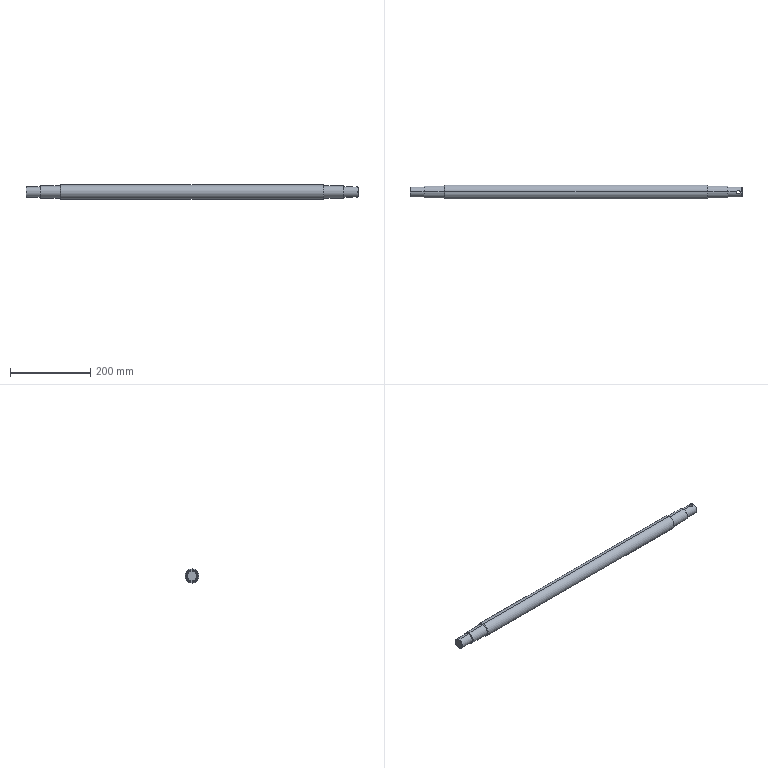Part | SolidWorks | features BaseBody 1 | 1 solid | 30 faces | box 825 x 35 x 35 mm | volume 733390 mm3 | cylinder 12 | cone 12 | plane 6 | commonest cylinder face diameters 25 x4 30 x4 9 x2 35 x2
STEP:
#1=CARTESIAN_POINT('',(86.,0.,-17.5));
#2=VERTEX_POINT('',#1);
#3=CARTESIAN_POINT('',(86.,0.,17.5));
#4=VERTEX_POINT('',#3);
#5=CARTESIAN_POINT('',(86.,0.,0.));
#6=DIRECTION('',(1.,0.,0.));
#7=DIRECTION('',(0.,0.,-1.));
#8=AXIS2_PLACEMENT_3D('',#5,#6,#7);
#9=CIRCLE('',#8,17.5);
#10=EDGE_CURVE('',#2,#4,#9,.T.);
#11=ORIENTED_EDGE('',*,*,#10,.T.);
#12=CARTESIAN_POINT('',(739.,0.,17.5));
#13=VERTEX_POINT('',#12);
#14=CARTESIAN_POINT('',(412.5,0.,17.5));
#15=DIRECTION('',(1.,0.,0.));
#16=VECTOR('',#15,1000.);
#17=LINE('',#14,#16);
#18=EDGE_CURVE('',#4,#13,#17,.T.);
#19=ORIENTED_EDGE('',*,*,#18,.T.);
#20=CARTESIAN_POINT('',(739.,0.,-17.5));
#21=VERTEX_POINT('',#20);
#22=CARTESIAN_POINT('',(739.,0.,0.));
#23=DIRECTION('',(-1.,0.,0.));
#24=DIRECTION('',(0.,0.,-1.));
#25=AXIS2_PLACEMENT_3D('',#22,#23,#24);
#26=CIRCLE('',#25,17.5);
#27=EDGE_CURVE('',#13,#21,#26,.T.);
#28=ORIENTED_EDGE('',*,*,#27,.T.);
#29=CARTESIAN_POINT('',(412.5,0.,-17.5));
#30=DIRECTION('',(1.,0.,0.));
#31=VECTOR('',#30,1000.);
#32=LINE('',#29,#31);
#33=EDGE_CURVE('',#2,#21,#32,.T.);
#34=ORIENTED_EDGE('',*,*,#33,.F.);
#35=EDGE_LOOP('',(#11,#19,#28,#34));
#36=FACE_OUTER_BOUND('',#35,.T.);
#37=CARTESIAN_POINT('',(412.5,0.,0.));
#38=DIRECTION('',(1.,0.,0.));
#39=DIRECTION('',(0.,0.,-1.));
#40=AXIS2_PLACEMENT_3D('',#37,#38,#39);
#41=CYLINDRICAL_SURFACE('',#40,17.5);
#42=ADVANCED_FACE('',(#36),#41,.T.);
#43=CARTESIAN_POINT('',(740.,0.,16.5));
#44=VERTEX_POINT('',#43);
#45=CARTESIAN_POINT('',(740.,0.,-16.5));
#46=VERTEX_POINT('',#45);
#47=CARTESIAN_POINT('',(740.,0.,0.));
#48=DIRECTION('',(-1.,0.,0.));
#49=DIRECTION('',(0.,0.,1.));
#50=AXIS2_PLACEMENT_3D('',#47,#48,#49);
#51=CIRCLE('',#50,16.5);
#52=EDGE_CURVE('',#44,#46,#51,.T.);
#53=ORIENTED_EDGE('',*,*,#52,.T.);
#54=CARTESIAN_POINT('',(739.,0.,-17.5));
#55=DIRECTION('',(-0.7071,0.,-0.7071));
#56=VECTOR('',#55,1000.);
#57=LINE('',#54,#56);
#58=EDGE_CURVE('',#46,#21,#57,.T.);
#59=ORIENTED_EDGE('',*,*,#58,.T.);
#60=ORIENTED_EDGE('',*,*,#27,.F.);
#61=CARTESIAN_POINT('',(739.,0.,17.5));
#62=DIRECTION('',(-0.7071,0.,0.7071));
#63=VECTOR('',#62,1000.);
#64=LINE('',#61,#63);
#65=EDGE_CURVE('',#44,#13,#64,.T.);
#66=ORIENTED_EDGE('',*,*,#65,.F.);
#67=EDGE_LOOP('',(#53,#59,#60,#66));
#68=FACE_OUTER_BOUND('',#67,.T.);
#69=CARTESIAN_POINT('',(739.,0.,0.));
#70=DIRECTION('',(-1.,0.,0.));
#71=DIRECTION('',(0.,0.,1.));
#72=AXIS2_PLACEMENT_3D('',#69,#70,#71);
#73=CONICAL_SURFACE('',#72,17.5,0.7854);
#74=ADVANCED_FACE('',(#68),#73,.T.);
#75=CARTESIAN_POINT('',(85.,0.,-16.5));
#76=VERTEX_POINT('',#75);
#77=CARTESIAN_POINT('',(85.,0.,16.5));
#78=VERTEX_POINT('',#77);
#79=CARTESIAN_POINT('',(85.,0.,0.));
#80=DIRECTION('',(1.,0.,0.));
#81=DIRECTION('',(0.,0.,-1.));
#82=AXIS2_PLACEMENT_3D('',#79,#80,#81);
#83=CIRCLE('',#82,16.5);
#84=EDGE_CURVE('',#76,#78,#83,.T.);
#85=ORIENTED_EDGE('',*,*,#84,.T.);
#86=CARTESIAN_POINT('',(86.,0.,17.5));
#87=DIRECTION('',(0.7071,0.,0.7071));
#88=VECTOR('',#87,1000.);
#89=LINE('',#86,#88);
#90=EDGE_CURVE('',#78,#4,#89,.T.);
#91=ORIENTED_EDGE('',*,*,#90,.T.);
#92=ORIENTED_EDGE('',*,*,#10,.F.);
#93=CARTESIAN_POINT('',(86.,0.,-17.5));
#94=DIRECTION('',(0.7071,0.,-0.7071));
#95=VECTOR('',#94,1000.);
#96=LINE('',#93,#95);
#97=EDGE_CURVE('',#76,#2,#96,.T.);
#98=ORIENTED_EDGE('',*,*,#97,.F.);
#99=EDGE_LOOP('',(#85,#91,#92,#98));
#100=FACE_OUTER_BOUND('',#99,.T.);
#101=CARTESIAN_POINT('',(86.,0.,0.));
#102=DIRECTION('',(1.,0.,0.));
#103=DIRECTION('',(0.,0.,-1.));
#104=AXIS2_PLACEMENT_3D('',#101,#102,#103);
#105=CONICAL_SURFACE('',#104,17.5,0.7854);
#106=ADVANCED_FACE('',(#100),#105,.T.);
#107=CARTESIAN_POINT('',(740.,0.,15.));
#108=VERTEX_POINT('',#107);
#109=CARTESIAN_POINT('',(740.,0.,-15.));
#110=VERTEX_POINT('',#109);
#111=CARTESIAN_POINT('',(740.,0.,0.));
#112=DIRECTION('',(-1.,0.,0.));
#113=DIRECTION('',(0.,0.,-1.));
#114=AXIS2_PLACEMENT_3D('',#111,#112,#113);
#115=CIRCLE('',#114,15.);
#116=EDGE_CURVE('',#108,#110,#115,.T.);
#117=ORIENTED_EDGE('',*,*,#116,.F.);
#118=CARTESIAN_POINT('',(789.,0.,15.));
#119=VERTEX_POINT('',#118);
#120=CARTESIAN_POINT('',(765.,0.,15.));
#121=DIRECTION('',(1.,0.,0.));
#122=VECTOR('',#121,1000.);
#123=LINE('',#120,#122);
#124=EDGE_CURVE('',#108,#119,#123,.T.);
#125=ORIENTED_EDGE('',*,*,#124,.T.);
#126=CARTESIAN_POINT('',(789.,0.,-15.));
#127=VERTEX_POINT('',#126);
#128=CARTESIAN_POINT('',(789.,0.,0.));
#129=DIRECTION('',(-1.,0.,0.));
#130=DIRECTION('',(0.,0.,-1.));
#131=AXIS2_PLACEMENT_3D('',#128,#129,#130);
#132=CIRCLE('',#131,15.);
#133=EDGE_CURVE('',#119,#127,#132,.T.);
#134=ORIENTED_EDGE('',*,*,#133,.T.);
#135=CARTESIAN_POINT('',(765.,0.,-15.));
#136=DIRECTION('',(1.,0.,0.));
#137=VECTOR('',#136,1000.);
#138=LINE('',#135,#137);
#139=EDGE_CURVE('',#110,#127,#138,.T.);
#140=ORIENTED_EDGE('',*,*,#139,.F.);
#141=EDGE_LOOP('',(#117,#125,#134,#140));
#142=FACE_OUTER_BOUND('',#141,.T.);
#143=CARTESIAN_POINT('',(765.,0.,0.));
#144=DIRECTION('',(1.,0.,0.));
#145=DIRECTION('',(0.,0.,-1.));
#146=AXIS2_PLACEMENT_3D('',#143,#144,#145);
#147=CYLINDRICAL_SURFACE('',#146,15.);
#148=ADVANCED_FACE('',(#142),#147,.T.);
#149=CARTESIAN_POINT('',(36.,0.,-15.));
#150=VERTEX_POINT('',#149);
#151=CARTESIAN_POINT('',(36.,0.,15.));
#152=VERTEX_POINT('',#151);
#153=CARTESIAN_POINT('',(36.,0.,0.));
#154=DIRECTION('',(1.,0.,0.));
#155=DIRECTION('',(0.,0.,-1.));
#156=AXIS2_PLACEMENT_3D('',#153,#154,#155);
#157=CIRCLE('',#156,15.);
#158=EDGE_CURVE('',#150,#152,#157,.T.);
#159=ORIENTED_EDGE('',*,*,#158,.T.);
#160=CARTESIAN_POINT('',(85.,0.,15.));
#161=VERTEX_POINT('',#160);
#162=CARTESIAN_POINT('',(60.,0.,15.));
#163=DIRECTION('',(1.,0.,0.));
#164=VECTOR('',#163,1000.);
#165=LINE('',#162,#164);
#166=EDGE_CURVE('',#152,#161,#165,.T.);
#167=ORIENTED_EDGE('',*,*,#166,.T.);
#168=CARTESIAN_POINT('',(85.,0.,-15.));
#169=VERTEX_POINT('',#168);
#170=CARTESIAN_POINT('',(85.,0.,0.));
#171=DIRECTION('',(1.,0.,0.));
#172=DIRECTION('',(0.,0.,-1.));
#173=AXIS2_PLACEMENT_3D('',#170,#171,#172);
#174=CIRCLE('',#173,15.);
#175=EDGE_CURVE('',#169,#161,#174,.T.);
#176=ORIENTED_EDGE('',*,*,#175,.F.);
#177=CARTESIAN_POINT('',(60.,0.,-15.));
#178=DIRECTION('',(1.,0.,0.));
#179=VECTOR('',#178,1000.);
#180=LINE('',#177,#179);
#181=EDGE_CURVE('',#150,#169,#180,.T.);
#182=ORIENTED_EDGE('',*,*,#181,.F.);
#183=EDGE_LOOP('',(#159,#167,#176,#182));
#184=FACE_OUTER_BOUND('',#183,.T.);
#185=CARTESIAN_POINT('',(60.,0.,0.));
#186=DIRECTION('',(1.,0.,0.));
#187=DIRECTION('',(0.,0.,-1.));
#188=AXIS2_PLACEMENT_3D('',#185,#186,#187);
#189=CYLINDRICAL_SURFACE('',#188,15.);
#190=ADVANCED_FACE('',(#184),#189,.T.);
#191=CARTESIAN_POINT('',(790.,0.,14.));
#192=VERTEX_POINT('',#191);
#193=CARTESIAN_POINT('',(790.,0.,-14.));
#194=VERTEX_POINT('',#193);
#195=CARTESIAN_POINT('',(790.,0.,0.));
#196=DIRECTION('',(-1.,0.,0.));
#197=DIRECTION('',(0.,0.,1.));
#198=AXIS2_PLACEMENT_3D('',#195,#196,#197);
#199=CIRCLE('',#198,14.);
#200=EDGE_CURVE('',#192,#194,#199,.T.);
#201=ORIENTED_EDGE('',*,*,#200,.T.);
#202=CARTESIAN_POINT('',(789.,0.,-15.));
#203=DIRECTION('',(-0.7071,0.,-0.7071));
#204=VECTOR('',#203,1000.);
#205=LINE('',#202,#204);
#206=EDGE_CURVE('',#194,#127,#205,.T.);
#207=ORIENTED_EDGE('',*,*,#206,.T.);
#208=ORIENTED_EDGE('',*,*,#133,.F.);
#209=CARTESIAN_POINT('',(789.,0.,15.));
#210=DIRECTION('',(-0.7071,0.,0.7071));
#211=VECTOR('',#210,1000.);
#212=LINE('',#209,#211);
#213=EDGE_CURVE('',#192,#119,#212,.T.);
#214=ORIENTED_EDGE('',*,*,#213,.F.);
#215=EDGE_LOOP('',(#201,#207,#208,#214));
#216=FACE_OUTER_BOUND('',#215,.T.);
#217=CARTESIAN_POINT('',(789.,0.,0.));
#218=DIRECTION('',(-1.,0.,0.));
#219=DIRECTION('',(0.,0.,1.));
#220=AXIS2_PLACEMENT_3D('',#217,#218,#219);
#221=CONICAL_SURFACE('',#220,15.,0.7854);
#222=ADVANCED_FACE('',(#216),#221,.T.);
#223=CARTESIAN_POINT('',(35.,0.,-14.));
#224=VERTEX_POINT('',#223);
#225=CARTESIAN_POINT('',(35.,0.,14.));
#226=VERTEX_POINT('',#225);
#227=CARTESIAN_POINT('',(35.,0.,0.));
#228=DIRECTION('',(1.,0.,0.));
#229=DIRECTION('',(0.,0.,-1.));
#230=AXIS2_PLACEMENT_3D('',#227,#228,#229);
#231=CIRCLE('',#230,14.);
#232=EDGE_CURVE('',#224,#226,#231,.T.);
#233=ORIENTED_EDGE('',*,*,#232,.T.);
#234=CARTESIAN_POINT('',(36.,0.,15.));
#235=DIRECTION('',(0.7071,0.,0.7071));
#236=VECTOR('',#235,1000.);
#237=LINE('',#234,#236);
#238=EDGE_CURVE('',#226,#152,#237,.T.);
#239=ORIENTED_EDGE('',*,*,#238,.T.);
#240=ORIENTED_EDGE('',*,*,#158,.F.);
#241=CARTESIAN_POINT('',(36.,0.,-15.));
#242=DIRECTION('',(0.7071,0.,-0.7071));
#243=VECTOR('',#242,1000.);
#244=LINE('',#241,#243);
#245=EDGE_CURVE('',#224,#150,#244,.T.);
#246=ORIENTED_EDGE('',*,*,#245,.F.);
#247=EDGE_LOOP('',(#233,#239,#240,#246));
#248=FACE_OUTER_BOUND('',#247,.T.);
#249=CARTESIAN_POINT('',(36.,0.,0.));
#250=DIRECTION('',(1.,0.,0.));
#251=DIRECTION('',(0.,0.,-1.));
#252=AXIS2_PLACEMENT_3D('',#249,#250,#251);
#253=CONICAL_SURFACE('',#252,15.,0.7854);
#254=ADVANCED_FACE('',(#248),#253,.T.);
#255=CARTESIAN_POINT('',(790.,0.,12.5));
#256=VERTEX_POINT('',#255);
#257=CARTESIAN_POINT('',(790.,0.,-12.5));
#258=VERTEX_POINT('',#257);
#259=CARTESIAN_POINT('',(790.,0.,0.));
#260=DIRECTION('',(-1.,0.,0.));
#261=DIRECTION('',(0.,0.,-1.));
#262=AXIS2_PLACEMENT_3D('',#259,#260,#261);
#263=CIRCLE('',#262,12.5);
#264=EDGE_CURVE('',#256,#258,#263,.T.);
#265=ORIENTED_EDGE('',*,*,#264,.F.);
#266=CARTESIAN_POINT('',(811.5,0.,12.5));
#267=VERTEX_POINT('',#266);
#268=CARTESIAN_POINT('',(807.5,0.,12.5));
#269=DIRECTION('',(1.,0.,0.));
#270=VECTOR('',#269,1000.);
#271=LINE('',#268,#270);
#272=EDGE_CURVE('',#256,#267,#271,.T.);
#273=ORIENTED_EDGE('',*,*,#272,.T.);
#274=CARTESIAN_POINT('',(820.5,0.,12.5));
#275=VERTEX_POINT('',#274);
#276=CARTESIAN_POINT('',(811.5,0.,12.5));
#277=CARTESIAN_POINT('',(811.5,0.2964,12.5));
#278=CARTESIAN_POINT('',(811.53,0.5972,12.489));
#279=CARTESIAN_POINT('',(811.646,1.176,12.448));
#280=CARTESIAN_POINT('',(811.732,1.458,12.418));
#281=CARTESIAN_POINT('',(811.961,2.006,12.341));
#282=CARTESIAN_POINT('',(812.101,2.265,12.296));
#283=CARTESIAN_POINT('',(812.426,2.75,12.196));
#284=CARTESIAN_POINT('',(812.614,2.979,12.142));
#285=CARTESIAN_POINT('',(813.028,3.391,12.033));
#286=CARTESIAN_POINT('',(813.252,3.576,11.979));
#287=CARTESIAN_POINT('',(813.738,3.901,11.877));
#288=CARTESIAN_POINT('',(814.001,4.042,11.829));
#289=CARTESIAN_POINT('',(814.542,4.267,11.75));
#290=CARTESIAN_POINT('',(814.823,4.353,11.718));
#291=CARTESIAN_POINT('',(815.406,4.471,11.673));
#292=CARTESIAN_POINT('',(815.704,4.5,11.662));
#293=CARTESIAN_POINT('',(816.295,4.5,11.662));
#294=CARTESIAN_POINT('',(816.593,4.471,11.673));
#295=CARTESIAN_POINT('',(817.176,4.354,11.717));
#296=CARTESIAN_POINT('',(817.458,4.267,11.75));
#297=CARTESIAN_POINT('',(818.001,4.041,11.829));
#298=CARTESIAN_POINT('',(818.264,3.9,11.877));
#299=CARTESIAN_POINT('',(818.749,3.575,11.979));
#300=CARTESIAN_POINT('',(818.974,3.39,12.033));
#301=CARTESIAN_POINT('',(819.39,2.974,12.143));
#302=CARTESIAN_POINT('',(819.575,2.748,12.197));
#303=CARTESIAN_POINT('',(819.9,2.264,12.296));
#304=CARTESIAN_POINT('',(820.041,2.003,12.342));
#305=CARTESIAN_POINT('',(820.268,1.457,12.418));
#306=CARTESIAN_POINT('',(820.354,1.176,12.448));
#307=CARTESIAN_POINT('',(820.47,0.5975,12.489));
#308=CARTESIAN_POINT('',(820.5,0.2965,12.5));
#309=CARTESIAN_POINT('',(820.5,0.,12.5));
#310=B_SPLINE_CURVE_WITH_KNOTS('',3,(#276,#277,#278,#279,#280,#281,#282,#283,#284,#285,#286,#287,#288,#289,#290,#291,#292,#293,#294,#295,#296,#297,#298,#299,#300,#301,#302,#303,#304,#305,#306,#307,#308,#309),.UNSPECIFIED.,.F.,.F.,(4,2,2,2,2,2,2,2,2,2,2,2,2,2,2,2,4),(0.007097,0.007983,0.008869,0.009756,0.01064,0.01153,0.01242,0.0133,0.01419,0.01507,0.01596,0.01685,0.01773,0.01862,0.01951,0.02039,0.02128),.UNSPECIFIED.);
#311=EDGE_CURVE('',#267,#275,#310,.T.);
#312=ORIENTED_EDGE('',*,*,#311,.T.);
#313=CARTESIAN_POINT('',(824.,0.,12.5));
#314=VERTEX_POINT('',#313);
#315=CARTESIAN_POINT('',(807.5,0.,12.5));
#316=DIRECTION('',(1.,0.,0.));
#317=VECTOR('',#316,1000.);
#318=LINE('',#315,#317);
#319=EDGE_CURVE('',#275,#314,#318,.T.);
#320=ORIENTED_EDGE('',*,*,#319,.T.);
#321=CARTESIAN_POINT('',(824.,0.,-12.5));
#322=VERTEX_POINT('',#321);
#323=CARTESIAN_POINT('',(824.,0.,0.));
#324=DIRECTION('',(-1.,0.,0.));
#325=DIRECTION('',(0.,0.,-1.));
#326=AXIS2_PLACEMENT_3D('',#323,#324,#325);
#327=CIRCLE('',#326,12.5);
#328=EDGE_CURVE('',#314,#322,#327,.T.);
#329=ORIENTED_EDGE('',*,*,#328,.T.);
#330=CARTESIAN_POINT('',(820.5,0.,-12.5));
#331=VERTEX_POINT('',#330);
#332=CARTESIAN_POINT('',(807.5,0.,-12.5));
#333=DIRECTION('',(1.,0.,0.));
#334=VECTOR('',#333,1000.);
#335=LINE('',#332,#334);
#336=EDGE_CURVE('',#331,#322,#335,.T.);
#337=ORIENTED_EDGE('',*,*,#336,.F.);
#338=CARTESIAN_POINT('',(811.5,0.,-12.5));
#339=VERTEX_POINT('',#338);
#340=CARTESIAN_POINT('',(820.5,0.,-12.5));
#341=CARTESIAN_POINT('',(820.5,0.2964,-12.5));
#342=CARTESIAN_POINT('',(820.47,0.5972,-12.489));
#343=CARTESIAN_POINT('',(820.354,1.176,-12.448));
#344=CARTESIAN_POINT('',(820.268,1.458,-12.418));
#345=CARTESIAN_POINT('',(820.039,2.006,-12.341));
#346=CARTESIAN_POINT('',(819.899,2.265,-12.296));
#347=CARTESIAN_POINT('',(819.574,2.75,-12.196));
#348=CARTESIAN_POINT('',(819.386,2.979,-12.142));
#349=CARTESIAN_POINT('',(818.972,3.391,-12.033));
#350=CARTESIAN_POINT('',(818.748,3.576,-11.979));
#351=CARTESIAN_POINT('',(818.262,3.901,-11.877));
#352=CARTESIAN_POINT('',(817.999,4.042,-11.829));
#353=CARTESIAN_POINT('',(817.458,4.267,-11.75));
#354=CARTESIAN_POINT('',(817.177,4.353,-11.718));
#355=CARTESIAN_POINT('',(816.594,4.471,-11.673));
#356=CARTESIAN_POINT('',(816.296,4.5,-11.662));
#357=CARTESIAN_POINT('',(815.705,4.5,-11.662));
#358=CARTESIAN_POINT('',(815.407,4.471,-11.673));
#359=CARTESIAN_POINT('',(814.824,4.354,-11.717));
#360=CARTESIAN_POINT('',(814.542,4.267,-11.75));
#361=CARTESIAN_POINT('',(813.999,4.041,-11.829));
#362=CARTESIAN_POINT('',(813.736,3.9,-11.877));
#363=CARTESIAN_POINT('',(813.251,3.575,-11.979));
#364=CARTESIAN_POINT('',(813.026,3.39,-12.033));
#365=CARTESIAN_POINT('',(812.61,2.974,-12.143));
#366=CARTESIAN_POINT('',(812.425,2.748,-12.197));
#367=CARTESIAN_POINT('',(812.1,2.264,-12.296));
#368=CARTESIAN_POINT('',(811.959,2.003,-12.342));
#369=CARTESIAN_POINT('',(811.732,1.457,-12.418));
#370=CARTESIAN_POINT('',(811.646,1.176,-12.448));
#371=CARTESIAN_POINT('',(811.53,0.5975,-12.489));
#372=CARTESIAN_POINT('',(811.5,0.2965,-12.5));
#373=CARTESIAN_POINT('',(811.5,0.,-12.5));
#374=B_SPLINE_CURVE_WITH_KNOTS('',3,(#340,#341,#342,#343,#344,#345,#346,#347,#348,#349,#350,#351,#352,#353,#354,#355,#356,#357,#358,#359,#360,#361,#362,#363,#364,#365,#366,#367,#368,#369,#370,#371,#372,#373),.UNSPECIFIED.,.F.,.F.,(4,2,2,2,2,2,2,2,2,2,2,2,2,2,2,2,4),(0.007097,0.007983,0.008869,0.009756,0.01064,0.01153,0.01242,0.0133,0.01419,0.01507,0.01596,0.01685,0.01773,0.01862,0.01951,0.02039,0.02128),.UNSPECIFIED.);
#375=EDGE_CURVE('',#331,#339,#374,.T.);
#376=ORIENTED_EDGE('',*,*,#375,.T.);
#377=CARTESIAN_POINT('',(807.5,0.,-12.5));
#378=DIRECTION('',(1.,0.,0.));
#379=VECTOR('',#378,1000.);
#380=LINE('',#377,#379);
#381=EDGE_CURVE('',#258,#339,#380,.T.);
#382=ORIENTED_EDGE('',*,*,#381,.F.);
#383=EDGE_LOOP('',(#265,#273,#312,#320,#329,#337,#376,#382));
#384=FACE_OUTER_BOUND('',#383,.T.);
#385=CARTESIAN_POINT('',(807.5,0.,0.));
#386=DIRECTION('',(1.,0.,0.));
#387=DIRECTION('',(0.,0.,-1.));
#388=AXIS2_PLACEMENT_3D('',#385,#386,#387);
#389=CYLINDRICAL_SURFACE('',#388,12.5);
#390=ADVANCED_FACE('',(#384),#389,.T.);
#391=CARTESIAN_POINT('',(1.,0.,-12.5));
#392=VERTEX_POINT('',#391);
#393=CARTESIAN_POINT('',(1.,0.,12.5));
#394=VERTEX_POINT('',#393);
#395=CARTESIAN_POINT('',(1.,0.,0.));
#396=DIRECTION('',(1.,0.,0.));
#397=DIRECTION('',(0.,0.,-1.));
#398=AXIS2_PLACEMENT_3D('',#395,#396,#397);
#399=CIRCLE('',#398,12.5);
#400=EDGE_CURVE('',#392,#394,#399,.T.);
#401=ORIENTED_EDGE('',*,*,#400,.T.);
#402=CARTESIAN_POINT('',(35.,0.,12.5));
#403=VERTEX_POINT('',#402);
#404=CARTESIAN_POINT('',(17.5,0.,12.5));
#405=DIRECTION('',(1.,0.,0.));
#406=VECTOR('',#405,1000.);
#407=LINE('',#404,#406);
#408=EDGE_CURVE('',#394,#403,#407,.T.);
#409=ORIENTED_EDGE('',*,*,#408,.T.);
#410=CARTESIAN_POINT('',(35.,0.,-12.5));
#411=VERTEX_POINT('',#410);
#412=CARTESIAN_POINT('',(35.,0.,0.));
#413=DIRECTION('',(1.,0.,0.));
#414=DIRECTION('',(0.,0.,-1.));
#415=AXIS2_PLACEMENT_3D('',#412,#413,#414);
#416=CIRCLE('',#415,12.5);
#417=EDGE_CURVE('',#411,#403,#416,.T.);
#418=ORIENTED_EDGE('',*,*,#417,.F.);
#419=CARTESIAN_POINT('',(17.5,0.,-12.5));
#420=DIRECTION('',(1.,0.,0.));
#421=VECTOR('',#420,1000.);
#422=LINE('',#419,#421);
#423=EDGE_CURVE('',#392,#411,#422,.T.);
#424=ORIENTED_EDGE('',*,*,#423,.F.);
#425=EDGE_LOOP('',(#401,#409,#418,#424));
#426=FACE_OUTER_BOUND('',#425,.T.);
#427=CARTESIAN_POINT('',(17.5,0.,0.));
#428=DIRECTION('',(1.,0.,0.));
#429=DIRECTION('',(0.,0.,-1.));
#430=AXIS2_PLACEMENT_3D('',#427,#428,#429);
#431=CYLINDRICAL_SURFACE('',#430,12.5);
#432=ADVANCED_FACE('',(#426),#431,.T.);
#433=CARTESIAN_POINT('',(825.,0.,11.5));
#434=VERTEX_POINT('',#433);
#435=CARTESIAN_POINT('',(825.,0.,-11.5));
#436=VERTEX_POINT('',#435);
#437=CARTESIAN_POINT('',(825.,0.,0.));
#438=DIRECTION('',(-1.,0.,0.));
#439=DIRECTION('',(0.,0.,1.));
#440=AXIS2_PLACEMENT_3D('',#437,#438,#439);
#441=CIRCLE('',#440,11.5);
#442=EDGE_CURVE('',#434,#436,#441,.T.);
#443=ORIENTED_EDGE('',*,*,#442,.T.);
#444=CARTESIAN_POINT('',(824.,0.,-12.5));
#445=DIRECTION('',(-0.7071,0.,-0.7071));
#446=VECTOR('',#445,1000.);
#447=LINE('',#444,#446);
#448=EDGE_CURVE('',#436,#322,#447,.T.);
#449=ORIENTED_EDGE('',*,*,#448,.T.);
#450=ORIENTED_EDGE('',*,*,#328,.F.);
#451=CARTESIAN_POINT('',(824.,0.,12.5));
#452=DIRECTION('',(-0.7071,0.,0.7071));
#453=VECTOR('',#452,1000.);
#454=LINE('',#451,#453);
#455=EDGE_CURVE('',#434,#314,#454,.T.);
#456=ORIENTED_EDGE('',*,*,#455,.F.);
#457=EDGE_LOOP('',(#443,#449,#450,#456));
#458=FACE_OUTER_BOUND('',#457,.T.);
#459=CARTESIAN_POINT('',(824.,0.,0.));
#460=DIRECTION('',(-1.,0.,0.));
#461=DIRECTION('',(0.,0.,1.));
#462=AXIS2_PLACEMENT_3D('',#459,#460,#461);
#463=CONICAL_SURFACE('',#462,12.5,0.7854);
#464=ADVANCED_FACE('',(#458),#463,.T.);
#465=CARTESIAN_POINT('',(811.5,0.,-12.5));
#466=CARTESIAN_POINT('',(811.5,-0.2966,-12.5));
#467=CARTESIAN_POINT('',(811.529,-0.5909,-12.489));
#468=CARTESIAN_POINT('',(811.646,-1.174,-12.448));
#469=CARTESIAN_POINT('',(811.733,-1.46,-12.417));
#470=CARTESIAN_POINT('',(811.959,-2.002,-12.342));
#471=CARTESIAN_POINT('',(812.1,-2.264,-12.296));
#472=CARTESIAN_POINT('',(812.428,-2.752,-12.196));
#473=CARTESIAN_POINT('',(812.613,-2.977,-12.142));
#474=CARTESIAN_POINT('',(813.026,-3.39,-12.034));
#475=CARTESIAN_POINT('',(813.256,-3.578,-11.978));
#476=CARTESIAN_POINT('',(813.741,-3.903,-11.876));
#477=CARTESIAN_POINT('',(813.998,-4.041,-11.829));
#478=CARTESIAN_POINT('',(814.407,-4.211,-11.769));
#479=CARTESIAN_POINT('',(814.548,-4.262,-11.751));
#480=CARTESIAN_POINT('',(814.831,-4.348,-11.72));
#481=CARTESIAN_POINT('',(814.974,-4.384,-11.706));
#482=CARTESIAN_POINT('',(815.407,-4.47,-11.673));
#483=CARTESIAN_POINT('',(815.701,-4.5,-11.662));
#484=CARTESIAN_POINT('',(816.301,-4.5,-11.662));
#485=CARTESIAN_POINT('',(816.596,-4.47,-11.674));
#486=CARTESIAN_POINT('',(817.174,-4.354,-11.717));
#487=CARTESIAN_POINT('',(817.461,-4.266,-11.75));
#488=CARTESIAN_POINT('',(818.005,-4.039,-11.83));
#489=CARTESIAN_POINT('',(818.262,-3.901,-11.877));
#490=CARTESIAN_POINT('',(818.75,-3.574,-11.979));
#491=CARTESIAN_POINT('',(818.978,-3.386,-12.034));
#492=CARTESIAN_POINT('',(819.389,-2.975,-12.143));
#493=CARTESIAN_POINT('',(819.575,-2.749,-12.197));
#494=CARTESIAN_POINT('',(819.904,-2.258,-12.297));
#495=CARTESIAN_POINT('',(820.042,-2.,-12.342));
#496=CARTESIAN_POINT('',(820.211,-1.594,-12.399));
#497=CARTESIAN_POINT('',(820.261,-1.456,-12.416));
#498=CARTESIAN_POINT('',(820.347,-1.173,-12.446));
#499=CARTESIAN_POINT('',(820.384,-1.027,-12.459));
#500=CARTESIAN_POINT('',(820.471,-0.5904,-12.489));
#501=CARTESIAN_POINT('',(820.5,-0.2965,-12.5));
#502=CARTESIAN_POINT('',(820.5,0.,-12.5));
#503=B_SPLINE_CURVE_WITH_KNOTS('',3,(#465,#466,#467,#468,#469,#470,#471,#472,#473,#474,#475,#476,#477,#478,#479,#480,#481,#482,#483,#484,#485,#486,#487,#488,#489,#490,#491,#492,#493,#494,#495,#496,#497,#498,#499,#500,#501,#502),.UNSPECIFIED.,.F.,.F.,(4,2,2,2,2,2,2,2,2,2,2,2,2,2,2,2,2,2,4),(0.02128,0.02217,0.02305,0.02394,0.02483,0.02571,0.0266,0.02704,0.02749,0.02838,0.02926,0.03015,0.03104,0.03192,0.03281,0.0337,0.03414,0.03458,0.03547),.UNSPECIFIED.);
#504=EDGE_CURVE('',#339,#331,#503,.T.);
#505=ORIENTED_EDGE('',*,*,#504,.F.);
#506=CARTESIAN_POINT('',(811.5,0.,0.));
#507=DIRECTION('',(0.,0.,1.));
#508=VECTOR('',#507,1000.);
#509=LINE('',#506,#508);
#510=EDGE_CURVE('',#339,#267,#509,.T.);
#511=ORIENTED_EDGE('',*,*,#510,.T.);
#512=CARTESIAN_POINT('',(820.5,0.,12.5));
#513=CARTESIAN_POINT('',(820.5,-0.2966,12.5));
#514=CARTESIAN_POINT('',(820.471,-0.5909,12.489));
#515=CARTESIAN_POINT('',(820.354,-1.174,12.448));
#516=CARTESIAN_POINT('',(820.267,-1.46,12.417));
#517=CARTESIAN_POINT('',(820.041,-2.002,12.342));
#518=CARTESIAN_POINT('',(819.9,-2.264,12.296));
#519=CARTESIAN_POINT('',(819.572,-2.752,12.196));
#520=CARTESIAN_POINT('',(819.387,-2.977,12.142));
#521=CARTESIAN_POINT('',(818.974,-3.39,12.034));
#522=CARTESIAN_POINT('',(818.744,-3.578,11.978));
#523=CARTESIAN_POINT('',(818.259,-3.903,11.876));
#524=CARTESIAN_POINT('',(818.002,-4.041,11.829));
#525=CARTESIAN_POINT('',(817.593,-4.211,11.769));
#526=CARTESIAN_POINT('',(817.452,-4.262,11.751));
#527=CARTESIAN_POINT('',(817.169,-4.348,11.72));
#528=CARTESIAN_POINT('',(817.026,-4.384,11.706));
#529=CARTESIAN_POINT('',(816.593,-4.47,11.673));
#530=CARTESIAN_POINT('',(816.299,-4.5,11.662));
#531=CARTESIAN_POINT('',(815.699,-4.5,11.662));
#532=CARTESIAN_POINT('',(815.404,-4.47,11.674));
#533=CARTESIAN_POINT('',(814.826,-4.354,11.717));
#534=CARTESIAN_POINT('',(814.539,-4.266,11.75));
#535=CARTESIAN_POINT('',(813.995,-4.039,11.83));
#536=CARTESIAN_POINT('',(813.738,-3.901,11.877));
#537=CARTESIAN_POINT('',(813.25,-3.574,11.979));
#538=CARTESIAN_POINT('',(813.022,-3.386,12.034));
#539=CARTESIAN_POINT('',(812.611,-2.975,12.143));
#540=CARTESIAN_POINT('',(812.425,-2.749,12.197));
#541=CARTESIAN_POINT('',(812.096,-2.258,12.297));
#542=CARTESIAN_POINT('',(811.958,-2.,12.342));
#543=CARTESIAN_POINT('',(811.789,-1.594,12.399));
#544=CARTESIAN_POINT('',(811.739,-1.456,12.416));
#545=CARTESIAN_POINT('',(811.653,-1.173,12.446));
#546=CARTESIAN_POINT('',(811.616,-1.027,12.459));
#547=CARTESIAN_POINT('',(811.529,-0.5904,12.489));
#548=CARTESIAN_POINT('',(811.5,-0.2965,12.5));
#549=CARTESIAN_POINT('',(811.5,0.,12.5));
#550=B_SPLINE_CURVE_WITH_KNOTS('',3,(#512,#513,#514,#515,#516,#517,#518,#519,#520,#521,#522,#523,#524,#525,#526,#527,#528,#529,#530,#531,#532,#533,#534,#535,#536,#537,#538,#539,#540,#541,#542,#543,#544,#545,#546,#547,#548,#549),.UNSPECIFIED.,.F.,.F.,(4,2,2,2,2,2,2,2,2,2,2,2,2,2,2,2,2,2,4),(0.02128,0.02217,0.02305,0.02394,0.02483,0.02571,0.0266,0.02704,0.02749,0.02838,0.02926,0.03015,0.03104,0.03192,0.03281,0.0337,0.03414,0.03458,0.03547),.UNSPECIFIED.);
#551=EDGE_CURVE('',#275,#267,#550,.T.);
#552=ORIENTED_EDGE('',*,*,#551,.F.);
#553=CARTESIAN_POINT('',(820.5,0.,0.));
#554=DIRECTION('',(0.,0.,1.));
#555=VECTOR('',#554,1000.);
#556=LINE('',#553,#555);
#557=EDGE_CURVE('',#331,#275,#556,.T.);
#558=ORIENTED_EDGE('',*,*,#557,.F.);
#559=EDGE_LOOP('',(#505,#511,#552,#558));
#560=FACE_OUTER_BOUND('',#559,.T.);
#561=CARTESIAN_POINT('',(816.,0.,0.));
#562=DIRECTION('',(0.,0.,1.));
#563=DIRECTION('',(1.,0.,0.));
#564=AXIS2_PLACEMENT_3D('',#561,#562,#563);
#565=CYLINDRICAL_SURFACE('',#564,4.5);
#566=ADVANCED_FACE('',(#560),#565,.F.);
#567=CARTESIAN_POINT('',(0.,0.,-11.5));
#568=VERTEX_POINT('',#567);
#569=CARTESIAN_POINT('',(0.,0.,11.5));
#570=VERTEX_POINT('',#569);
#571=CARTESIAN_POINT('',(0.,0.,0.));
#572=DIRECTION('',(1.,0.,0.));
#573=DIRECTION('',(0.,0.,-1.));
#574=AXIS2_PLACEMENT_3D('',#571,#572,#573);
#575=CIRCLE('',#574,11.5);
#576=EDGE_CURVE('',#568,#570,#575,.T.);
#577=ORIENTED_EDGE('',*,*,#576,.T.);
#578=CARTESIAN_POINT('',(1.,0.,12.5));
#579=DIRECTION('',(0.7071,0.,0.7071));
#580=VECTOR('',#579,1000.);
#581=LINE('',#578,#580);
#582=EDGE_CURVE('',#570,#394,#581,.T.);
#583=ORIENTED_EDGE('',*,*,#582,.T.);
#584=ORIENTED_EDGE('',*,*,#400,.F.);
#585=CARTESIAN_POINT('',(1.,0.,-12.5));
#586=DIRECTION('',(0.7071,0.,-0.7071));
#587=VECTOR('',#586,1000.);
#588=LINE('',#585,#587);
#589=EDGE_CURVE('',#568,#392,#588,.T.);
#590=ORIENTED_EDGE('',*,*,#589,.F.);
#591=EDGE_LOOP('',(#577,#583,#584,#590));
#592=FACE_OUTER_BOUND('',#591,.T.);
#593=CARTESIAN_POINT('',(1.,0.,0.));
#594=DIRECTION('',(1.,0.,0.));
#595=DIRECTION('',(0.,0.,-1.));
#596=AXIS2_PLACEMENT_3D('',#593,#594,#595);
#597=CONICAL_SURFACE('',#596,12.5,0.7854);
#598=ADVANCED_FACE('',(#592),#597,.T.);
#599=ORIENTED_EDGE('',*,*,#18,.F.);
#600=CARTESIAN_POINT('',(86.,0.,0.));
#601=DIRECTION('',(1.,0.,0.));
#602=DIRECTION('',(0.,0.,-1.));
#603=AXIS2_PLACEMENT_3D('',#600,#601,#602);
#604=CIRCLE('',#603,17.5);
#605=EDGE_CURVE('',#4,#2,#604,.T.);
#606=ORIENTED_EDGE('',*,*,#605,.T.);
#607=ORIENTED_EDGE('',*,*,#33,.T.);
#608=CARTESIAN_POINT('',(739.,0.,0.));
#609=DIRECTION('',(-1.,0.,0.));
#610=DIRECTION('',(0.,0.,-1.));
#611=AXIS2_PLACEMENT_3D('',#608,#609,#610);
#612=CIRCLE('',#611,17.5);
#613=EDGE_CURVE('',#21,#13,#612,.T.);
#614=ORIENTED_EDGE('',*,*,#613,.T.);
#615=EDGE_LOOP('',(#599,#606,#607,#614));
#616=FACE_OUTER_BOUND('',#615,.T.);
#617=CARTESIAN_POINT('',(412.5,0.,0.));
#618=DIRECTION('',(1.,0.,0.));
#619=DIRECTION('',(0.,0.,-1.));
#620=AXIS2_PLACEMENT_3D('',#617,#618,#619);
#621=CYLINDRICAL_SURFACE('',#620,17.5);
#622=ADVANCED_FACE('',(#616),#621,.T.);
#623=ORIENTED_EDGE('',*,*,#58,.F.);
#624=CARTESIAN_POINT('',(740.,0.,0.));
#625=DIRECTION('',(-1.,0.,0.));
#626=DIRECTION('',(0.,0.,1.));
#627=AXIS2_PLACEMENT_3D('',#624,#625,#626);
#628=CIRCLE('',#627,16.5);
#629=EDGE_CURVE('',#46,#44,#628,.T.);
#630=ORIENTED_EDGE('',*,*,#629,.T.);
#631=ORIENTED_EDGE('',*,*,#65,.T.);
#632=ORIENTED_EDGE('',*,*,#613,.F.);
#633=EDGE_LOOP('',(#623,#630,#631,#632));
#634=FACE_OUTER_BOUND('',#633,.T.);
#635=CARTESIAN_POINT('',(739.,0.,0.));
#636=DIRECTION('',(-1.,0.,0.));
#637=DIRECTION('',(0.,0.,1.));
#638=AXIS2_PLACEMENT_3D('',#635,#636,#637);
#639=CONICAL_SURFACE('',#638,17.5,0.7854);
#640=ADVANCED_FACE('',(#634),#639,.T.);
#641=ORIENTED_EDGE('',*,*,#90,.F.);
#642=CARTESIAN_POINT('',(85.,0.,0.));
#643=DIRECTION('',(1.,0.,0.));
#644=DIRECTION('',(0.,0.,-1.));
#645=AXIS2_PLACEMENT_3D('',#642,#643,#644);
#646=CIRCLE('',#645,16.5);
#647=EDGE_CURVE('',#78,#76,#646,.T.);
#648=ORIENTED_EDGE('',*,*,#647,.T.);
#649=ORIENTED_EDGE('',*,*,#97,.T.);
#650=ORIENTED_EDGE('',*,*,#605,.F.);
#651=EDGE_LOOP('',(#641,#648,#649,#650));
#652=FACE_OUTER_BOUND('',#651,.T.);
#653=CARTESIAN_POINT('',(86.,0.,0.));
#654=DIRECTION('',(1.,0.,0.));
#655=DIRECTION('',(0.,0.,-1.));
#656=AXIS2_PLACEMENT_3D('',#653,#654,#655);
#657=CONICAL_SURFACE('',#656,17.5,0.7854);
#658=ADVANCED_FACE('',(#652),#657,.T.);
#659=CARTESIAN_POINT('',(740.,0.,0.));
#660=DIRECTION('',(-1.,0.,0.));
#661=DIRECTION('',(0.,0.,-1.));
#662=AXIS2_PLACEMENT_3D('',#659,#660,#661);
#663=CIRCLE('',#662,15.);
#664=EDGE_CURVE('',#110,#108,#663,.T.);
#665=ORIENTED_EDGE('',*,*,#664,.T.);
#666=ORIENTED_EDGE('',*,*,#116,.T.);
#667=EDGE_LOOP('',(#665,#666));
#668=FACE_BOUND('',#667,.T.);
#669=ORIENTED_EDGE('',*,*,#52,.F.);
#670=ORIENTED_EDGE('',*,*,#629,.F.);
#671=EDGE_LOOP('',(#669,#670));
#672=FACE_OUTER_BOUND('',#671,.T.);
#673=CARTESIAN_POINT('',(740.,15.,0.));
#674=DIRECTION('',(1.,0.,0.));
#675=DIRECTION('',(0.,0.,-1.));
#676=AXIS2_PLACEMENT_3D('',#673,#674,#675);
#677=PLANE('',#676);
#678=ADVANCED_FACE('',(#668,#672),#677,.T.);
#679=ORIENTED_EDGE('',*,*,#175,.T.);
#680=CARTESIAN_POINT('',(85.,0.,0.));
#681=DIRECTION('',(1.,0.,0.));
#682=DIRECTION('',(0.,0.,-1.));
#683=AXIS2_PLACEMENT_3D('',#680,#681,#682);
#684=CIRCLE('',#683,15.);
#685=EDGE_CURVE('',#161,#169,#684,.T.);
#686=ORIENTED_EDGE('',*,*,#685,.T.);
#687=EDGE_LOOP('',(#679,#686));
#688=FACE_BOUND('',#687,.T.);
#689=ORIENTED_EDGE('',*,*,#84,.F.);
#690=ORIENTED_EDGE('',*,*,#647,.F.);
#691=EDGE_LOOP('',(#689,#690));
#692=FACE_OUTER_BOUND('',#691,.T.);
#693=CARTESIAN_POINT('',(85.,17.5,0.));
#694=DIRECTION('',(-1.,0.,0.));
#695=DIRECTION('',(0.,0.,1.));
#696=AXIS2_PLACEMENT_3D('',#693,#694,#695);
#697=PLANE('',#696);
#698=ADVANCED_FACE('',(#688,#692),#697,.T.);
#699=ORIENTED_EDGE('',*,*,#124,.F.);
#700=ORIENTED_EDGE('',*,*,#664,.F.);
#701=ORIENTED_EDGE('',*,*,#139,.T.);
#702=CARTESIAN_POINT('',(789.,0.,0.));
#703=DIRECTION('',(-1.,0.,0.));
#704=DIRECTION('',(0.,0.,-1.));
#705=AXIS2_PLACEMENT_3D('',#702,#703,#704);
#706=CIRCLE('',#705,15.);
#707=EDGE_CURVE('',#127,#119,#706,.T.);
#708=ORIENTED_EDGE('',*,*,#707,.T.);
#709=EDGE_LOOP('',(#699,#700,#701,#708));
#710=FACE_OUTER_BOUND('',#709,.T.);
#711=CARTESIAN_POINT('',(765.,0.,0.));
#712=DIRECTION('',(1.,0.,0.));
#713=DIRECTION('',(0.,0.,-1.));
#714=AXIS2_PLACEMENT_3D('',#711,#712,#713);
#715=CYLINDRICAL_SURFACE('',#714,15.);
#716=ADVANCED_FACE('',(#710),#715,.T.);
#717=ORIENTED_EDGE('',*,*,#166,.F.);
#718=CARTESIAN_POINT('',(36.,0.,0.));
#719=DIRECTION('',(1.,0.,0.));
#720=DIRECTION('',(0.,0.,-1.));
#721=AXIS2_PLACEMENT_3D('',#718,#719,#720);
#722=CIRCLE('',#721,15.);
#723=EDGE_CURVE('',#152,#150,#722,.T.);
#724=ORIENTED_EDGE('',*,*,#723,.T.);
#725=ORIENTED_EDGE('',*,*,#181,.T.);
#726=ORIENTED_EDGE('',*,*,#685,.F.);
#727=EDGE_LOOP('',(#717,#724,#725,#726));
#728=FACE_OUTER_BOUND('',#727,.T.);
#729=CARTESIAN_POINT('',(60.,0.,0.));
#730=DIRECTION('',(1.,0.,0.));
#731=DIRECTION('',(0.,0.,-1.));
#732=AXIS2_PLACEMENT_3D('',#729,#730,#731);
#733=CYLINDRICAL_SURFACE('',#732,15.);
#734=ADVANCED_FACE('',(#728),#733,.T.);
#735=ORIENTED_EDGE('',*,*,#206,.F.);
#736=CARTESIAN_POINT('',(790.,0.,0.));
#737=DIRECTION('',(-1.,0.,0.));
#738=DIRECTION('',(0.,0.,1.));
#739=AXIS2_PLACEMENT_3D('',#736,#737,#738);
#740=CIRCLE('',#739,14.);
#741=EDGE_CURVE('',#194,#192,#740,.T.);
#742=ORIENTED_EDGE('',*,*,#741,.T.);
#743=ORIENTED_EDGE('',*,*,#213,.T.);
#744=ORIENTED_EDGE('',*,*,#707,.F.);
#745=EDGE_LOOP('',(#735,#742,#743,#744));
#746=FACE_OUTER_BOUND('',#745,.T.);
#747=CARTESIAN_POINT('',(789.,0.,0.));
#748=DIRECTION('',(-1.,0.,0.));
#749=DIRECTION('',(0.,0.,1.));
#750=AXIS2_PLACEMENT_3D('',#747,#748,#749);
#751=CONICAL_SURFACE('',#750,15.,0.7854);
#752=ADVANCED_FACE('',(#746),#751,.T.);
#753=ORIENTED_EDGE('',*,*,#238,.F.);
#754=CARTESIAN_POINT('',(35.,0.,0.));
#755=DIRECTION('',(1.,0.,0.));
#756=DIRECTION('',(0.,0.,-1.));
#757=AXIS2_PLACEMENT_3D('',#754,#755,#756);
#758=CIRCLE('',#757,14.);
#759=EDGE_CURVE('',#226,#224,#758,.T.);
#760=ORIENTED_EDGE('',*,*,#759,.T.);
#761=ORIENTED_EDGE('',*,*,#245,.T.);
#762=ORIENTED_EDGE('',*,*,#723,.F.);
#763=EDGE_LOOP('',(#753,#760,#761,#762));
#764=FACE_OUTER_BOUND('',#763,.T.);
#765=CARTESIAN_POINT('',(36.,0.,0.));
#766=DIRECTION('',(1.,0.,0.));
#767=DIRECTION('',(0.,0.,-1.));
#768=AXIS2_PLACEMENT_3D('',#765,#766,#767);
#769=CONICAL_SURFACE('',#768,15.,0.7854);
#770=ADVANCED_FACE('',(#764),#769,.T.);
#771=CARTESIAN_POINT('',(790.,0.,0.));
#772=DIRECTION('',(-1.,0.,0.));
#773=DIRECTION('',(0.,0.,-1.));
#774=AXIS2_PLACEMENT_3D('',#771,#772,#773);
#775=CIRCLE('',#774,12.5);
#776=EDGE_CURVE('',#258,#256,#775,.T.);
#777=ORIENTED_EDGE('',*,*,#776,.T.);
#778=ORIENTED_EDGE('',*,*,#264,.T.);
#779=EDGE_LOOP('',(#777,#778));
#780=FACE_BOUND('',#779,.T.);
#781=ORIENTED_EDGE('',*,*,#200,.F.);
#782=ORIENTED_EDGE('',*,*,#741,.F.);
#783=EDGE_LOOP('',(#781,#782));
#784=FACE_OUTER_BOUND('',#783,.T.);
#785=CARTESIAN_POINT('',(790.,12.5,0.));
#786=DIRECTION('',(1.,0.,0.));
#787=DIRECTION('',(0.,0.,-1.));
#788=AXIS2_PLACEMENT_3D('',#785,#786,#787);
#789=PLANE('',#788);
#790=ADVANCED_FACE('',(#780,#784),#789,.T.);
#791=ORIENTED_EDGE('',*,*,#417,.T.);
#792=CARTESIAN_POINT('',(35.,0.,0.));
#793=DIRECTION('',(1.,0.,0.));
#794=DIRECTION('',(0.,0.,-1.));
#795=AXIS2_PLACEMENT_3D('',#792,#793,#794);
#796=CIRCLE('',#795,12.5);
#797=EDGE_CURVE('',#403,#411,#796,.T.);
#798=ORIENTED_EDGE('',*,*,#797,.T.);
#799=EDGE_LOOP('',(#791,#798));
#800=FACE_BOUND('',#799,.T.);
#801=ORIENTED_EDGE('',*,*,#232,.F.);
#802=ORIENTED_EDGE('',*,*,#759,.F.);
#803=EDGE_LOOP('',(#801,#802));
#804=FACE_OUTER_BOUND('',#803,.T.);
#805=CARTESIAN_POINT('',(35.,15.,0.));
#806=DIRECTION('',(-1.,0.,0.));
#807=DIRECTION('',(0.,0.,1.));
#808=AXIS2_PLACEMENT_3D('',#805,#806,#807);
#809=PLANE('',#808);
#810=ADVANCED_FACE('',(#800,#804),#809,.T.);
#811=ORIENTED_EDGE('',*,*,#272,.F.);
#812=ORIENTED_EDGE('',*,*,#776,.F.);
#813=ORIENTED_EDGE('',*,*,#381,.T.);
#814=ORIENTED_EDGE('',*,*,#504,.T.);
#815=ORIENTED_EDGE('',*,*,#336,.T.);
#816=CARTESIAN_POINT('',(824.,0.,0.));
#817=DIRECTION('',(-1.,0.,0.));
#818=DIRECTION('',(0.,0.,-1.));
#819=AXIS2_PLACEMENT_3D('',#816,#817,#818);
#820=CIRCLE('',#819,12.5);
#821=EDGE_CURVE('',#322,#314,#820,.T.);
#822=ORIENTED_EDGE('',*,*,#821,.T.);
#823=ORIENTED_EDGE('',*,*,#319,.F.);
#824=ORIENTED_EDGE('',*,*,#551,.T.);
#825=EDGE_LOOP('',(#811,#812,#813,#814,#815,#822,#823,#824));
#826=FACE_OUTER_BOUND('',#825,.T.);
#827=CARTESIAN_POINT('',(807.5,0.,0.));
#828=DIRECTION('',(1.,0.,0.));
#829=DIRECTION('',(0.,0.,-1.));
#830=AXIS2_PLACEMENT_3D('',#827,#828,#829);
#831=CYLINDRICAL_SURFACE('',#830,12.5);
#832=ADVANCED_FACE('',(#826),#831,.T.);
#833=ORIENTED_EDGE('',*,*,#408,.F.);
#834=CARTESIAN_POINT('',(1.,0.,0.));
#835=DIRECTION('',(1.,0.,0.));
#836=DIRECTION('',(0.,0.,-1.));
#837=AXIS2_PLACEMENT_3D('',#834,#835,#836);
#838=CIRCLE('',#837,12.5);
#839=EDGE_CURVE('',#394,#392,#838,.T.);
#840=ORIENTED_EDGE('',*,*,#839,.T.);
#841=ORIENTED_EDGE('',*,*,#423,.T.);
#842=ORIENTED_EDGE('',*,*,#797,.F.);
#843=EDGE_LOOP('',(#833,#840,#841,#842));
#844=FACE_OUTER_BOUND('',#843,.T.);
#845=CARTESIAN_POINT('',(17.5,0.,0.));
#846=DIRECTION('',(1.,0.,0.));
#847=DIRECTION('',(0.,0.,-1.));
#848=AXIS2_PLACEMENT_3D('',#845,#846,#847);
#849=CYLINDRICAL_SURFACE('',#848,12.5);
#850=ADVANCED_FACE('',(#844),#849,.T.);
#851=ORIENTED_EDGE('',*,*,#448,.F.);
#852=CARTESIAN_POINT('',(825.,0.,0.));
#853=DIRECTION('',(-1.,0.,0.));
#854=DIRECTION('',(0.,0.,1.));
#855=AXIS2_PLACEMENT_3D('',#852,#853,#854);
#856=CIRCLE('',#855,11.5);
#857=EDGE_CURVE('',#436,#434,#856,.T.);
#858=ORIENTED_EDGE('',*,*,#857,.T.);
#859=ORIENTED_EDGE('',*,*,#455,.T.);
#860=ORIENTED_EDGE('',*,*,#821,.F.);
#861=EDGE_LOOP('',(#851,#858,#859,#860));
#862=FACE_OUTER_BOUND('',#861,.T.);
#863=CARTESIAN_POINT('',(824.,0.,0.));
#864=DIRECTION('',(-1.,0.,0.));
#865=DIRECTION('',(0.,0.,1.));
#866=AXIS2_PLACEMENT_3D('',#863,#864,#865);
#867=CONICAL_SURFACE('',#866,12.5,0.7854);
#868=ADVANCED_FACE('',(#862),#867,.T.);
#869=ORIENTED_EDGE('',*,*,#510,.F.);
#870=ORIENTED_EDGE('',*,*,#375,.F.);
#871=ORIENTED_EDGE('',*,*,#557,.T.);
#872=ORIENTED_EDGE('',*,*,#311,.F.);
#873=EDGE_LOOP('',(#869,#870,#871,#872));
#874=FACE_OUTER_BOUND('',#873,.T.);
#875=CARTESIAN_POINT('',(816.,0.,0.));
#876=DIRECTION('',(0.,0.,1.));
#877=DIRECTION('',(1.,0.,0.));
#878=AXIS2_PLACEMENT_3D('',#875,#876,#877);
#879=CYLINDRICAL_SURFACE('',#878,4.5);
#880=ADVANCED_FACE('',(#874),#879,.F.);
#881=ORIENTED_EDGE('',*,*,#582,.F.);
#882=CARTESIAN_POINT('',(0.,0.,0.));
#883=DIRECTION('',(1.,0.,0.));
#884=DIRECTION('',(0.,0.,-1.));
#885=AXIS2_PLACEMENT_3D('',#882,#883,#884);
#886=CIRCLE('',#885,11.5);
#887=EDGE_CURVE('',#570,#568,#886,.T.);
#888=ORIENTED_EDGE('',*,*,#887,.T.);
#889=ORIENTED_EDGE('',*,*,#589,.T.);
#890=ORIENTED_EDGE('',*,*,#839,.F.);
#891=EDGE_LOOP('',(#881,#888,#889,#890));
#892=FACE_OUTER_BOUND('',#891,.T.);
#893=CARTESIAN_POINT('',(1.,0.,0.));
#894=DIRECTION('',(1.,0.,0.));
#895=DIRECTION('',(0.,0.,-1.));
#896=AXIS2_PLACEMENT_3D('',#893,#894,#895);
#897=CONICAL_SURFACE('',#896,12.5,0.7854);
#898=ADVANCED_FACE('',(#892),#897,.T.);
#899=ORIENTED_EDGE('',*,*,#442,.F.);
#900=ORIENTED_EDGE('',*,*,#857,.F.);
#901=EDGE_LOOP('',(#899,#900));
#902=FACE_OUTER_BOUND('',#901,.T.);
#903=CARTESIAN_POINT('',(825.,0.,0.));
#904=DIRECTION('',(1.,0.,0.));
#905=DIRECTION('',(0.,0.,-1.));
#906=AXIS2_PLACEMENT_3D('',#903,#904,#905);
#907=PLANE('',#906);
#908=ADVANCED_FACE('',(#902),#907,.T.);
#909=ORIENTED_EDGE('',*,*,#576,.F.);
#910=ORIENTED_EDGE('',*,*,#887,.F.);
#911=EDGE_LOOP('',(#909,#910));
#912=FACE_OUTER_BOUND('',#911,.T.);
#913=CARTESIAN_POINT('',(0.,12.5,0.));
#914=DIRECTION('',(-1.,0.,0.));
#915=DIRECTION('',(0.,0.,1.));
#916=AXIS2_PLACEMENT_3D('',#913,#914,#915);
#917=PLANE('',#916);
#918=ADVANCED_FACE('',(#912),#917,.T.);
#919=CLOSED_SHELL('',(#42,#74,#106,#148,#190,#222,#254,#390,#432,#464,#566,#598,#622,#640,#658,#678,#698,#716,#734,#752,#770,#790,#810,#832,#850,#868,#880,#898,#908,#918));
#920=MANIFOLD_SOLID_BREP('',#919);
#921=CARTESIAN_POINT('',(0.,0.,0.));
#922=DIRECTION('',(0.,0.,1.));
#923=DIRECTION('',(1.,0.,0.));
#924=AXIS2_PLACEMENT_3D('',#921,#922,#923);
#925=(LENGTH_UNIT()NAMED_UNIT(*)SI_UNIT(.MILLI.,.METRE.));
#926=UNCERTAINTY_MEASURE_WITH_UNIT(LENGTH_MEASURE(0.00001),#925,'','');
#927=(NAMED_UNIT(*)PLANE_ANGLE_UNIT()SI_UNIT($,.RADIAN.));
#928=(NAMED_UNIT(*)SI_UNIT($,.STERADIAN.)SOLID_ANGLE_UNIT());
#929=(GEOMETRIC_REPRESENTATION_CONTEXT(3)GLOBAL_UNCERTAINTY_ASSIGNED_CONTEXT((#926))GLOBAL_UNIT_ASSIGNED_CONTEXT((#925,#927,#928))REPRESENTATION_CONTEXT('',''));
#930=ADVANCED_BREP_SHAPE_REPRESENTATION('',(#920,#924),#929);